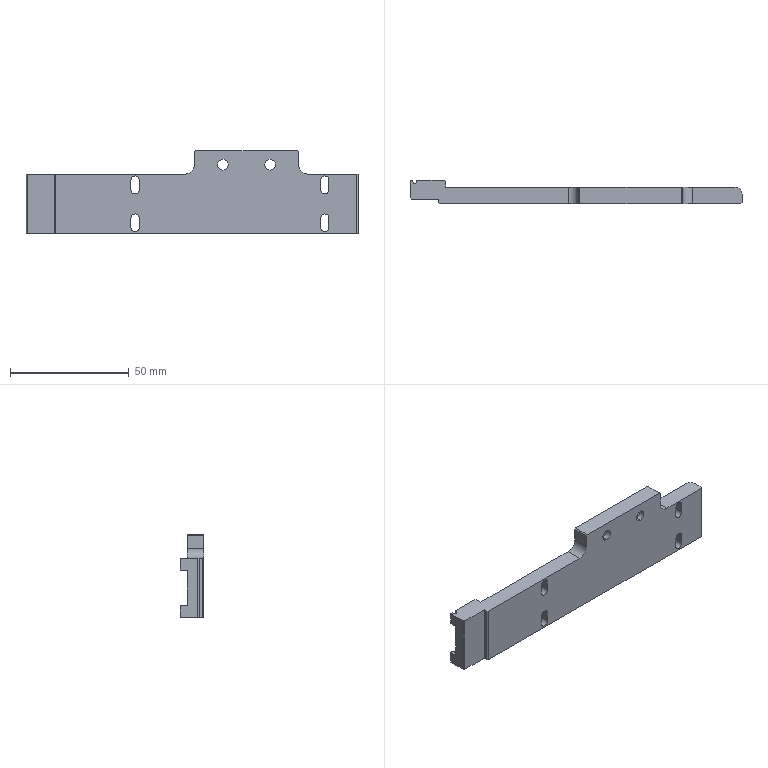Part | SolidWorks | features ICE 6, CutThin 5, HoleWzd 3, Emboss 2, Fillet 2, LPattern 2, MirrorPattern 2, Chamfer 1, Extrusion 1 | 1 solid | 410 faces | box 140 x 10 x 35 mm | volume 26170 mm3 | plane 345 | spline 32 | cylinder 29 | cone 4 | commonest cylinder face diameters 3.5 x12 8 x6 1.6 x4 4.5 x4 1.5 x2 6 x1